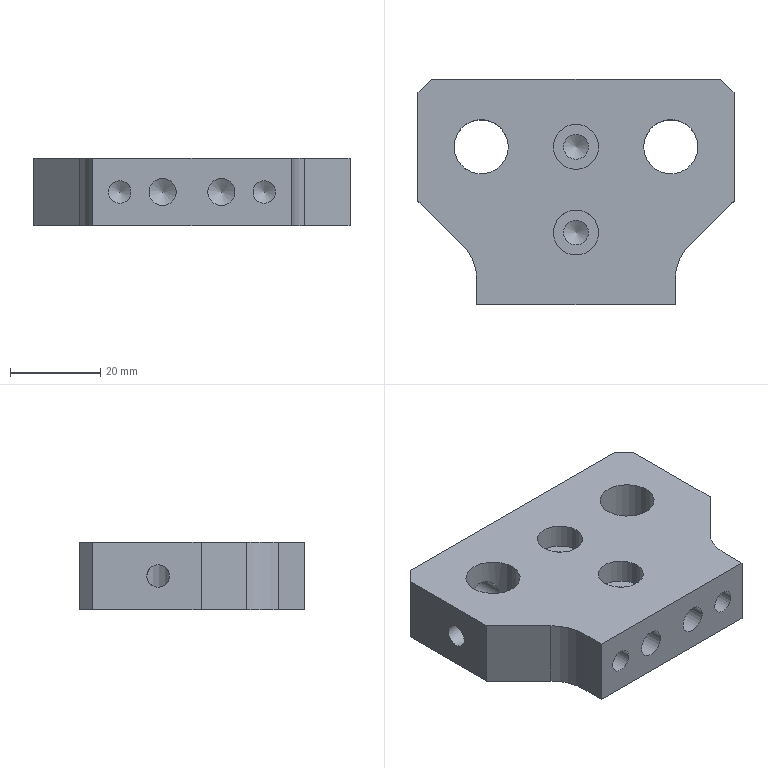Part | NX | features BREP 1 | 1 solid | 35 faces | box 70 x 50 x 15 mm | volume 39519 mm3 | cylinder 15 | plane 14 | cone 6 | commonest cylinder face diameters 5 x5 5.5 x2 6 x2 10 x2 12 x2 20 x2
STEP:
#1=CARTESIAN_POINT('',(35.,22.,0.));
#2=VERTEX_POINT('',#1);
#3=CARTESIAN_POINT('',(32.,25.,0.));
#4=VERTEX_POINT('',#3);
#5=CARTESIAN_POINT('',(35.,22.,0.));
#6=DIRECTION('',(-0.7071,0.7071,0.));
#7=VECTOR('',#6,1000.);
#8=LINE('',#5,#7);
#9=EDGE_CURVE('',#2,#4,#8,.T.);
#10=ORIENTED_EDGE('',*,*,#9,.F.);
#11=CARTESIAN_POINT('',(35.,-2.,0.));
#12=VERTEX_POINT('',#11);
#13=CARTESIAN_POINT('',(35.,0.,0.));
#14=DIRECTION('',(0.,1.,0.));
#15=VECTOR('',#14,1000.);
#16=LINE('',#13,#15);
#17=EDGE_CURVE('',#12,#2,#16,.T.);
#18=ORIENTED_EDGE('',*,*,#17,.F.);
#19=CARTESIAN_POINT('',(24.929,-12.071,0.));
#20=VERTEX_POINT('',#19);
#21=CARTESIAN_POINT('',(24.929,-12.071,0.));
#22=DIRECTION('',(0.7071,0.7071,0.));
#23=VECTOR('',#22,1000.);
#24=LINE('',#21,#23);
#25=EDGE_CURVE('',#20,#12,#24,.T.);
#26=ORIENTED_EDGE('',*,*,#25,.F.);
#27=CARTESIAN_POINT('',(22.,-19.142,0.));
#28=VERTEX_POINT('',#27);
#29=CARTESIAN_POINT('',(32.,-19.142,0.));
#30=DIRECTION('',(0.,0.,-1.));
#31=DIRECTION('',(1.,0.,0.));
#32=AXIS2_PLACEMENT_3D('',#29,#30,#31);
#33=CIRCLE('',#32,10.);
#34=EDGE_CURVE('',#28,#20,#33,.T.);
#35=ORIENTED_EDGE('',*,*,#34,.F.);
#36=CARTESIAN_POINT('',(22.,-25.,0.));
#37=VERTEX_POINT('',#36);
#38=CARTESIAN_POINT('',(22.,0.,0.));
#39=DIRECTION('',(0.,1.,0.));
#40=VECTOR('',#39,1000.);
#41=LINE('',#38,#40);
#42=EDGE_CURVE('',#37,#28,#41,.T.);
#43=ORIENTED_EDGE('',*,*,#42,.F.);
#44=CARTESIAN_POINT('',(-22.,-25.,0.));
#45=VERTEX_POINT('',#44);
#46=CARTESIAN_POINT('',(0.,-25.,0.));
#47=DIRECTION('',(1.,0.,0.));
#48=VECTOR('',#47,1000.);
#49=LINE('',#46,#48);
#50=EDGE_CURVE('',#45,#37,#49,.T.);
#51=ORIENTED_EDGE('',*,*,#50,.F.);
#52=CARTESIAN_POINT('',(-22.,-19.142,0.));
#53=VERTEX_POINT('',#52);
#54=CARTESIAN_POINT('',(-22.,0.,0.));
#55=DIRECTION('',(0.,-1.,0.));
#56=VECTOR('',#55,1000.);
#57=LINE('',#54,#56);
#58=EDGE_CURVE('',#53,#45,#57,.T.);
#59=ORIENTED_EDGE('',*,*,#58,.F.);
#60=CARTESIAN_POINT('',(-24.929,-12.071,0.));
#61=VERTEX_POINT('',#60);
#62=CARTESIAN_POINT('',(-32.,-19.142,0.));
#63=DIRECTION('',(0.,0.,-1.));
#64=DIRECTION('',(1.,0.,0.));
#65=AXIS2_PLACEMENT_3D('',#62,#63,#64);
#66=CIRCLE('',#65,10.);
#67=EDGE_CURVE('',#61,#53,#66,.T.);
#68=ORIENTED_EDGE('',*,*,#67,.F.);
#69=CARTESIAN_POINT('',(-35.,-2.,0.));
#70=VERTEX_POINT('',#69);
#71=CARTESIAN_POINT('',(-35.,-2.,0.));
#72=DIRECTION('',(0.7071,-0.7071,0.));
#73=VECTOR('',#72,1000.);
#74=LINE('',#71,#73);
#75=EDGE_CURVE('',#70,#61,#74,.T.);
#76=ORIENTED_EDGE('',*,*,#75,.F.);
#77=CARTESIAN_POINT('',(-35.,22.,0.));
#78=VERTEX_POINT('',#77);
#79=CARTESIAN_POINT('',(-35.,0.,0.));
#80=DIRECTION('',(0.,-1.,0.));
#81=VECTOR('',#80,1000.);
#82=LINE('',#79,#81);
#83=EDGE_CURVE('',#78,#70,#82,.T.);
#84=ORIENTED_EDGE('',*,*,#83,.F.);
#85=CARTESIAN_POINT('',(-32.,25.,0.));
#86=VERTEX_POINT('',#85);
#87=CARTESIAN_POINT('',(-32.,25.,0.));
#88=DIRECTION('',(-0.7071,-0.7071,0.));
#89=VECTOR('',#88,1000.);
#90=LINE('',#87,#89);
#91=EDGE_CURVE('',#86,#78,#90,.T.);
#92=ORIENTED_EDGE('',*,*,#91,.F.);
#93=CARTESIAN_POINT('',(0.,25.,0.));
#94=DIRECTION('',(-1.,0.,0.));
#95=VECTOR('',#94,1000.);
#96=LINE('',#93,#95);
#97=EDGE_CURVE('',#4,#86,#96,.T.);
#98=ORIENTED_EDGE('',*,*,#97,.F.);
#99=EDGE_LOOP('',(#10,#18,#26,#35,#43,#51,#59,#68,#76,#84,#92,#98));
#100=FACE_BOUND('',#99,.T.);
#101=CARTESIAN_POINT('',(15.,10.,0.));
#102=VERTEX_POINT('',#101);
#103=CARTESIAN_POINT('',(21.,10.,0.));
#104=DIRECTION('',(0.,0.,-1.));
#105=DIRECTION('',(-1.,0.,0.));
#106=AXIS2_PLACEMENT_3D('',#103,#104,#105);
#107=CIRCLE('',#106,6.);
#108=EDGE_CURVE('',#102,#102,#107,.T.);
#109=ORIENTED_EDGE('',*,*,#108,.F.);
#110=EDGE_LOOP('',(#109));
#111=FACE_BOUND('',#110,.T.);
#112=CARTESIAN_POINT('',(-27.,10.,0.));
#113=VERTEX_POINT('',#112);
#114=CARTESIAN_POINT('',(-21.,10.,0.));
#115=DIRECTION('',(0.,0.,-1.));
#116=DIRECTION('',(-1.,0.,0.));
#117=AXIS2_PLACEMENT_3D('',#114,#115,#116);
#118=CIRCLE('',#117,6.);
#119=EDGE_CURVE('',#113,#113,#118,.T.);
#120=ORIENTED_EDGE('',*,*,#119,.F.);
#121=EDGE_LOOP('',(#120));
#122=FACE_BOUND('',#121,.T.);
#123=CARTESIAN_POINT('',(0.,0.,0.));
#124=DIRECTION('',(0.,0.,1.));
#125=DIRECTION('',(-1.,0.,0.));
#126=AXIS2_PLACEMENT_3D('',#123,#124,#125);
#127=PLANE('',#126);
#128=ADVANCED_FACE('',(#100,#111,#122),#127,.F.);
#129=CARTESIAN_POINT('',(32.,25.,15.));
#130=VERTEX_POINT('',#129);
#131=CARTESIAN_POINT('',(32.,25.,15.));
#132=DIRECTION('',(0.,0.,1.));
#133=VECTOR('',#132,1000.);
#134=LINE('',#131,#133);
#135=EDGE_CURVE('',#4,#130,#134,.T.);
#136=ORIENTED_EDGE('',*,*,#135,.F.);
#137=ORIENTED_EDGE('',*,*,#97,.T.);
#138=CARTESIAN_POINT('',(-32.,25.,15.));
#139=VERTEX_POINT('',#138);
#140=CARTESIAN_POINT('',(-32.,25.,15.));
#141=DIRECTION('',(0.,0.,-1.));
#142=VECTOR('',#141,1000.);
#143=LINE('',#140,#142);
#144=EDGE_CURVE('',#139,#86,#143,.T.);
#145=ORIENTED_EDGE('',*,*,#144,.F.);
#146=CARTESIAN_POINT('',(-35.,25.,15.));
#147=DIRECTION('',(-1.,0.,0.));
#148=VECTOR('',#147,1000.);
#149=LINE('',#146,#148);
#150=EDGE_CURVE('',#130,#139,#149,.T.);
#151=ORIENTED_EDGE('',*,*,#150,.F.);
#152=EDGE_LOOP('',(#136,#137,#145,#151));
#153=FACE_BOUND('',#152,.T.);
#154=CARTESIAN_POINT('',(18.5,25.,10.));
#155=VERTEX_POINT('',#154);
#156=CARTESIAN_POINT('',(18.5,25.,7.5));
#157=DIRECTION('',(0.,1.,0.));
#158=DIRECTION('',(0.,0.,1.));
#159=AXIS2_PLACEMENT_3D('',#156,#157,#158);
#160=CIRCLE('',#159,2.5);
#161=EDGE_CURVE('',#155,#155,#160,.T.);
#162=ORIENTED_EDGE('',*,*,#161,.F.);
#163=EDGE_LOOP('',(#162));
#164=FACE_BOUND('',#163,.T.);
#165=CARTESIAN_POINT('',(-18.5,25.,10.));
#166=VERTEX_POINT('',#165);
#167=CARTESIAN_POINT('',(-18.5,25.,7.5));
#168=DIRECTION('',(0.,1.,0.));
#169=DIRECTION('',(0.,0.,1.));
#170=AXIS2_PLACEMENT_3D('',#167,#168,#169);
#171=CIRCLE('',#170,2.5);
#172=EDGE_CURVE('',#166,#166,#171,.T.);
#173=ORIENTED_EDGE('',*,*,#172,.F.);
#174=EDGE_LOOP('',(#173));
#175=FACE_BOUND('',#174,.T.);
#176=CARTESIAN_POINT('',(-35.,25.,15.));
#177=DIRECTION('',(0.,-1.,0.));
#178=DIRECTION('',(0.,0.,1.));
#179=AXIS2_PLACEMENT_3D('',#176,#177,#178);
#180=PLANE('',#179);
#181=ADVANCED_FACE('',(#153,#164,#175),#180,.F.);
#182=CARTESIAN_POINT('',(35.,22.,15.));
#183=VERTEX_POINT('',#182);
#184=CARTESIAN_POINT('',(35.,22.,15.));
#185=DIRECTION('',(0.,0.,1.));
#186=VECTOR('',#185,1000.);
#187=LINE('',#184,#186);
#188=EDGE_CURVE('',#2,#183,#187,.T.);
#189=ORIENTED_EDGE('',*,*,#188,.F.);
#190=ORIENTED_EDGE('',*,*,#9,.T.);
#191=ORIENTED_EDGE('',*,*,#135,.T.);
#192=CARTESIAN_POINT('',(32.,25.,15.));
#193=DIRECTION('',(-0.7071,0.7071,0.));
#194=VECTOR('',#193,1000.);
#195=LINE('',#192,#194);
#196=EDGE_CURVE('',#183,#130,#195,.T.);
#197=ORIENTED_EDGE('',*,*,#196,.F.);
#198=EDGE_LOOP('',(#189,#190,#191,#197));
#199=FACE_BOUND('',#198,.T.);
#200=CARTESIAN_POINT('',(32.,25.,15.));
#201=DIRECTION('',(-0.7071,-0.7071,0.));
#202=DIRECTION('',(-0.7071,0.7071,0.));
#203=AXIS2_PLACEMENT_3D('',#200,#201,#202);
#204=PLANE('',#203);
#205=ADVANCED_FACE('',(#199),#204,.F.);
#206=ORIENTED_EDGE('',*,*,#188,.T.);
#207=CARTESIAN_POINT('',(35.,-2.,15.));
#208=VERTEX_POINT('',#207);
#209=CARTESIAN_POINT('',(35.,25.,15.));
#210=DIRECTION('',(0.,1.,0.));
#211=VECTOR('',#210,1000.);
#212=LINE('',#209,#211);
#213=EDGE_CURVE('',#208,#183,#212,.T.);
#214=ORIENTED_EDGE('',*,*,#213,.F.);
#215=CARTESIAN_POINT('',(35.,-2.,15.));
#216=DIRECTION('',(0.,0.,1.));
#217=VECTOR('',#216,1000.);
#218=LINE('',#215,#217);
#219=EDGE_CURVE('',#12,#208,#218,.T.);
#220=ORIENTED_EDGE('',*,*,#219,.F.);
#221=ORIENTED_EDGE('',*,*,#17,.T.);
#222=EDGE_LOOP('',(#206,#214,#220,#221));
#223=FACE_BOUND('',#222,.T.);
#224=CARTESIAN_POINT('',(35.,25.,15.));
#225=DIRECTION('',(-1.,0.,0.));
#226=DIRECTION('',(0.,1.,0.));
#227=AXIS2_PLACEMENT_3D('',#224,#225,#226);
#228=PLANE('',#227);
#229=ADVANCED_FACE('',(#223),#228,.F.);
#230=CARTESIAN_POINT('',(24.929,-12.071,15.));
#231=VERTEX_POINT('',#230);
#232=CARTESIAN_POINT('',(24.929,-12.071,15.));
#233=DIRECTION('',(0.,0.,1.));
#234=VECTOR('',#233,1000.);
#235=LINE('',#232,#234);
#236=EDGE_CURVE('',#20,#231,#235,.T.);
#237=ORIENTED_EDGE('',*,*,#236,.F.);
#238=ORIENTED_EDGE('',*,*,#25,.T.);
#239=ORIENTED_EDGE('',*,*,#219,.T.);
#240=CARTESIAN_POINT('',(22.,-15.,15.));
#241=DIRECTION('',(0.7071,0.7071,0.));
#242=VECTOR('',#241,1000.);
#243=LINE('',#240,#242);
#244=EDGE_CURVE('',#231,#208,#243,.T.);
#245=ORIENTED_EDGE('',*,*,#244,.F.);
#246=EDGE_LOOP('',(#237,#238,#239,#245));
#247=FACE_BOUND('',#246,.T.);
#248=CARTESIAN_POINT('',(22.,-15.,15.));
#249=DIRECTION('',(-0.7071,0.7071,0.));
#250=DIRECTION('',(0.7071,0.7071,0.));
#251=AXIS2_PLACEMENT_3D('',#248,#249,#250);
#252=PLANE('',#251);
#253=ADVANCED_FACE('',(#247),#252,.F.);
#254=CARTESIAN_POINT('',(22.,-19.142,15.));
#255=VERTEX_POINT('',#254);
#256=CARTESIAN_POINT('',(22.,-19.142,15.));
#257=DIRECTION('',(0.,0.,1.));
#258=VECTOR('',#257,1000.);
#259=LINE('',#256,#258);
#260=EDGE_CURVE('',#28,#255,#259,.T.);
#261=ORIENTED_EDGE('',*,*,#260,.F.);
#262=ORIENTED_EDGE('',*,*,#34,.T.);
#263=ORIENTED_EDGE('',*,*,#236,.T.);
#264=CARTESIAN_POINT('',(32.,-19.142,15.));
#265=DIRECTION('',(0.,0.,-1.));
#266=DIRECTION('',(1.,0.,0.));
#267=AXIS2_PLACEMENT_3D('',#264,#265,#266);
#268=CIRCLE('',#267,10.);
#269=EDGE_CURVE('',#255,#231,#268,.T.);
#270=ORIENTED_EDGE('',*,*,#269,.F.);
#271=EDGE_LOOP('',(#261,#262,#263,#270));
#272=FACE_BOUND('',#271,.T.);
#273=CARTESIAN_POINT('',(32.,-19.142,15.));
#274=DIRECTION('',(0.,0.,1.));
#275=DIRECTION('',(-1.,0.,0.));
#276=AXIS2_PLACEMENT_3D('',#273,#274,#275);
#277=CYLINDRICAL_SURFACE('',#276,10.);
#278=ADVANCED_FACE('',(#272),#277,.F.);
#279=ORIENTED_EDGE('',*,*,#260,.T.);
#280=CARTESIAN_POINT('',(22.,-25.,15.));
#281=VERTEX_POINT('',#280);
#282=CARTESIAN_POINT('',(22.,-25.,15.));
#283=DIRECTION('',(0.,1.,0.));
#284=VECTOR('',#283,1000.);
#285=LINE('',#282,#284);
#286=EDGE_CURVE('',#281,#255,#285,.T.);
#287=ORIENTED_EDGE('',*,*,#286,.F.);
#288=CARTESIAN_POINT('',(22.,-25.,15.));
#289=DIRECTION('',(0.,0.,1.));
#290=VECTOR('',#289,1000.);
#291=LINE('',#288,#290);
#292=EDGE_CURVE('',#37,#281,#291,.T.);
#293=ORIENTED_EDGE('',*,*,#292,.F.);
#294=ORIENTED_EDGE('',*,*,#42,.T.);
#295=EDGE_LOOP('',(#279,#287,#293,#294));
#296=FACE_BOUND('',#295,.T.);
#297=CARTESIAN_POINT('',(22.,-25.,15.));
#298=DIRECTION('',(-1.,0.,0.));
#299=DIRECTION('',(0.,1.,0.));
#300=AXIS2_PLACEMENT_3D('',#297,#298,#299);
#301=PLANE('',#300);
#302=ADVANCED_FACE('',(#296),#301,.F.);
#303=ORIENTED_EDGE('',*,*,#50,.T.);
#304=ORIENTED_EDGE('',*,*,#292,.T.);
#305=CARTESIAN_POINT('',(-22.,-25.,15.));
#306=VERTEX_POINT('',#305);
#307=CARTESIAN_POINT('',(-35.,-25.,15.));
#308=DIRECTION('',(1.,0.,0.));
#309=VECTOR('',#308,1000.);
#310=LINE('',#307,#309);
#311=EDGE_CURVE('',#306,#281,#310,.T.);
#312=ORIENTED_EDGE('',*,*,#311,.F.);
#313=CARTESIAN_POINT('',(-22.,-25.,15.));
#314=DIRECTION('',(0.,0.,1.));
#315=VECTOR('',#314,1000.);
#316=LINE('',#313,#315);
#317=EDGE_CURVE('',#45,#306,#316,.T.);
#318=ORIENTED_EDGE('',*,*,#317,.F.);
#319=EDGE_LOOP('',(#303,#304,#312,#318));
#320=FACE_BOUND('',#319,.T.);
#321=CARTESIAN_POINT('',(16.,-25.,5.));
#322=VERTEX_POINT('',#321);
#323=CARTESIAN_POINT('',(16.,-25.,7.5));
#324=DIRECTION('',(0.,-1.,0.));
#325=DIRECTION('',(0.,0.,-1.));
#326=AXIS2_PLACEMENT_3D('',#323,#324,#325);
#327=CIRCLE('',#326,2.5);
#328=EDGE_CURVE('',#322,#322,#327,.T.);
#329=ORIENTED_EDGE('',*,*,#328,.F.);
#330=EDGE_LOOP('',(#329));
#331=FACE_BOUND('',#330,.T.);
#332=CARTESIAN_POINT('',(-16.,-25.,5.));
#333=VERTEX_POINT('',#332);
#334=CARTESIAN_POINT('',(-16.,-25.,7.5));
#335=DIRECTION('',(0.,-1.,0.));
#336=DIRECTION('',(0.,0.,-1.));
#337=AXIS2_PLACEMENT_3D('',#334,#335,#336);
#338=CIRCLE('',#337,2.5);
#339=EDGE_CURVE('',#333,#333,#338,.T.);
#340=ORIENTED_EDGE('',*,*,#339,.F.);
#341=EDGE_LOOP('',(#340));
#342=FACE_BOUND('',#341,.T.);
#343=CARTESIAN_POINT('',(6.5,-25.,4.5));
#344=VERTEX_POINT('',#343);
#345=CARTESIAN_POINT('',(6.5,-25.,7.5));
#346=DIRECTION('',(0.,-1.,0.));
#347=DIRECTION('',(0.,0.,-1.));
#348=AXIS2_PLACEMENT_3D('',#345,#346,#347);
#349=CIRCLE('',#348,3.);
#350=EDGE_CURVE('',#344,#344,#349,.T.);
#351=ORIENTED_EDGE('',*,*,#350,.F.);
#352=EDGE_LOOP('',(#351));
#353=FACE_BOUND('',#352,.T.);
#354=CARTESIAN_POINT('',(-6.5,-25.,4.5));
#355=VERTEX_POINT('',#354);
#356=CARTESIAN_POINT('',(-6.5,-25.,7.5));
#357=DIRECTION('',(0.,-1.,0.));
#358=DIRECTION('',(0.,0.,-1.));
#359=AXIS2_PLACEMENT_3D('',#356,#357,#358);
#360=CIRCLE('',#359,3.);
#361=EDGE_CURVE('',#355,#355,#360,.T.);
#362=ORIENTED_EDGE('',*,*,#361,.F.);
#363=EDGE_LOOP('',(#362));
#364=FACE_BOUND('',#363,.T.);
#365=CARTESIAN_POINT('',(-35.,-25.,15.));
#366=DIRECTION('',(0.,1.,0.));
#367=DIRECTION('',(0.,0.,-1.));
#368=AXIS2_PLACEMENT_3D('',#365,#366,#367);
#369=PLANE('',#368);
#370=ADVANCED_FACE('',(#320,#331,#342,#353,#364),#369,.F.);
#371=ORIENTED_EDGE('',*,*,#58,.T.);
#372=ORIENTED_EDGE('',*,*,#317,.T.);
#373=CARTESIAN_POINT('',(-22.,-19.142,15.));
#374=VERTEX_POINT('',#373);
#375=CARTESIAN_POINT('',(-22.,-25.,15.));
#376=DIRECTION('',(0.,1.,0.));
#377=VECTOR('',#376,1000.);
#378=LINE('',#375,#377);
#379=EDGE_CURVE('',#306,#374,#378,.T.);
#380=ORIENTED_EDGE('',*,*,#379,.T.);
#381=CARTESIAN_POINT('',(-22.,-19.142,15.));
#382=DIRECTION('',(0.,0.,-1.));
#383=VECTOR('',#382,1000.);
#384=LINE('',#381,#383);
#385=EDGE_CURVE('',#374,#53,#384,.T.);
#386=ORIENTED_EDGE('',*,*,#385,.T.);
#387=EDGE_LOOP('',(#371,#372,#380,#386));
#388=FACE_BOUND('',#387,.T.);
#389=CARTESIAN_POINT('',(-22.,-25.,15.));
#390=DIRECTION('',(-1.,0.,0.));
#391=DIRECTION('',(0.,1.,0.));
#392=AXIS2_PLACEMENT_3D('',#389,#390,#391);
#393=PLANE('',#392);
#394=ADVANCED_FACE('',(#388),#393,.T.);
#395=CARTESIAN_POINT('',(-24.929,-12.071,15.));
#396=VERTEX_POINT('',#395);
#397=CARTESIAN_POINT('',(-24.929,-12.071,15.));
#398=DIRECTION('',(0.,0.,1.));
#399=VECTOR('',#398,1000.);
#400=LINE('',#397,#399);
#401=EDGE_CURVE('',#61,#396,#400,.T.);
#402=ORIENTED_EDGE('',*,*,#401,.F.);
#403=ORIENTED_EDGE('',*,*,#67,.T.);
#404=ORIENTED_EDGE('',*,*,#385,.F.);
#405=CARTESIAN_POINT('',(-32.,-19.142,15.));
#406=DIRECTION('',(0.,0.,-1.));
#407=DIRECTION('',(1.,0.,0.));
#408=AXIS2_PLACEMENT_3D('',#405,#406,#407);
#409=CIRCLE('',#408,10.);
#410=EDGE_CURVE('',#396,#374,#409,.T.);
#411=ORIENTED_EDGE('',*,*,#410,.F.);
#412=EDGE_LOOP('',(#402,#403,#404,#411));
#413=FACE_BOUND('',#412,.T.);
#414=CARTESIAN_POINT('',(-32.,-19.142,15.));
#415=DIRECTION('',(0.,0.,1.));
#416=DIRECTION('',(-1.,0.,0.));
#417=AXIS2_PLACEMENT_3D('',#414,#415,#416);
#418=CYLINDRICAL_SURFACE('',#417,10.);
#419=ADVANCED_FACE('',(#413),#418,.F.);
#420=CARTESIAN_POINT('',(-35.,-2.,15.));
#421=VERTEX_POINT('',#420);
#422=CARTESIAN_POINT('',(-22.,-15.,15.));
#423=DIRECTION('',(-0.7071,0.7071,0.));
#424=VECTOR('',#423,1000.);
#425=LINE('',#422,#424);
#426=EDGE_CURVE('',#396,#421,#425,.T.);
#427=ORIENTED_EDGE('',*,*,#426,.T.);
#428=CARTESIAN_POINT('',(-35.,-2.,15.));
#429=DIRECTION('',(0.,0.,-1.));
#430=VECTOR('',#429,1000.);
#431=LINE('',#428,#430);
#432=EDGE_CURVE('',#421,#70,#431,.T.);
#433=ORIENTED_EDGE('',*,*,#432,.T.);
#434=ORIENTED_EDGE('',*,*,#75,.T.);
#435=ORIENTED_EDGE('',*,*,#401,.T.);
#436=EDGE_LOOP('',(#427,#433,#434,#435));
#437=FACE_BOUND('',#436,.T.);
#438=CARTESIAN_POINT('',(-22.,-15.,15.));
#439=DIRECTION('',(-0.7071,-0.7071,0.));
#440=DIRECTION('',(-0.7071,0.7071,0.));
#441=AXIS2_PLACEMENT_3D('',#438,#439,#440);
#442=PLANE('',#441);
#443=ADVANCED_FACE('',(#437),#442,.T.);
#444=CARTESIAN_POINT('',(-35.,22.,15.));
#445=VERTEX_POINT('',#444);
#446=CARTESIAN_POINT('',(-35.,22.,15.));
#447=DIRECTION('',(0.,0.,1.));
#448=VECTOR('',#447,1000.);
#449=LINE('',#446,#448);
#450=EDGE_CURVE('',#78,#445,#449,.T.);
#451=ORIENTED_EDGE('',*,*,#450,.F.);
#452=ORIENTED_EDGE('',*,*,#83,.T.);
#453=ORIENTED_EDGE('',*,*,#432,.F.);
#454=CARTESIAN_POINT('',(-35.,25.,15.));
#455=DIRECTION('',(0.,-1.,0.));
#456=VECTOR('',#455,1000.);
#457=LINE('',#454,#456);
#458=EDGE_CURVE('',#445,#421,#457,.T.);
#459=ORIENTED_EDGE('',*,*,#458,.F.);
#460=EDGE_LOOP('',(#451,#452,#453,#459));
#461=FACE_BOUND('',#460,.T.);
#462=CARTESIAN_POINT('',(-35.,7.5,10.));
#463=VERTEX_POINT('',#462);
#464=CARTESIAN_POINT('',(-35.,7.5,7.5));
#465=DIRECTION('',(-1.,0.,0.));
#466=DIRECTION('',(0.,0.,1.));
#467=AXIS2_PLACEMENT_3D('',#464,#465,#466);
#468=CIRCLE('',#467,2.5);
#469=EDGE_CURVE('',#463,#463,#468,.T.);
#470=ORIENTED_EDGE('',*,*,#469,.F.);
#471=EDGE_LOOP('',(#470));
#472=FACE_BOUND('',#471,.T.);
#473=CARTESIAN_POINT('',(-35.,25.,15.));
#474=DIRECTION('',(1.,0.,0.));
#475=DIRECTION('',(0.,-1.,0.));
#476=AXIS2_PLACEMENT_3D('',#473,#474,#475);
#477=PLANE('',#476);
#478=ADVANCED_FACE('',(#461,#472),#477,.F.);
#479=ORIENTED_EDGE('',*,*,#144,.T.);
#480=ORIENTED_EDGE('',*,*,#91,.T.);
#481=ORIENTED_EDGE('',*,*,#450,.T.);
#482=CARTESIAN_POINT('',(-35.,22.,15.));
#483=DIRECTION('',(-0.7071,-0.7071,0.));
#484=VECTOR('',#483,1000.);
#485=LINE('',#482,#484);
#486=EDGE_CURVE('',#139,#445,#485,.T.);
#487=ORIENTED_EDGE('',*,*,#486,.F.);
#488=EDGE_LOOP('',(#479,#480,#481,#487));
#489=FACE_BOUND('',#488,.T.);
#490=CARTESIAN_POINT('',(-35.,22.,15.));
#491=DIRECTION('',(0.7071,-0.7071,0.));
#492=DIRECTION('',(-0.7071,-0.7071,0.));
#493=AXIS2_PLACEMENT_3D('',#490,#491,#492);
#494=PLANE('',#493);
#495=ADVANCED_FACE('',(#489),#494,.F.);
#496=CARTESIAN_POINT('',(15.,10.,15.));
#497=VERTEX_POINT('',#496);
#498=CARTESIAN_POINT('',(21.,10.,15.));
#499=DIRECTION('',(0.,0.,-1.));
#500=DIRECTION('',(-1.,0.,0.));
#501=AXIS2_PLACEMENT_3D('',#498,#499,#500);
#502=CIRCLE('',#501,6.);
#503=EDGE_CURVE('',#497,#497,#502,.T.);
#504=ORIENTED_EDGE('',*,*,#503,.F.);
#505=EDGE_LOOP('',(#504));
#506=FACE_BOUND('',#505,.T.);
#507=CARTESIAN_POINT('',(18.5,15.454,5.));
#508=VERTEX_POINT('',#507);
#509=CARTESIAN_POINT('',(17.561,14.951,5.127));
#510=CARTESIAN_POINT('',(18.793,15.668,4.866));
#511=CARTESIAN_POINT('',(20.559,16.052,5.568));
#512=CARTESIAN_POINT('',(21.312,15.978,7.792));
#513=CARTESIAN_POINT('',(20.113,16.035,9.81));
#514=CARTESIAN_POINT('',(18.294,15.444,10.129));
#515=CARTESIAN_POINT('',(17.177,14.656,9.679));
#516=CARTESIAN_POINT('',(16.525,14.028,9.109));
#517=CARTESIAN_POINT('',(16.069,13.431,8.33));
#518=CARTESIAN_POINT('',(15.936,13.219,7.221));
#519=CARTESIAN_POINT('',(16.265,13.711,6.261));
#520=CARTESIAN_POINT('',(16.815,14.331,5.589));
#521=CARTESIAN_POINT('',(17.561,14.951,5.127));
#522=CARTESIAN_POINT('',(18.793,15.668,4.866));
#523=CARTESIAN_POINT('',(20.559,16.052,5.568));
#524=B_SPLINE_CURVE_WITH_KNOTS('',3,(#509,#510,#511,#512,#513,#514,#515,#516,#517,#518,#519,#520,#521,#522,#523),.UNSPECIFIED.,.T.,.F.,(1,1,1,1,1,1,1,1,1,1,1,1,1,1,1,1,1,1,1),(-0.00318,-0.00212,-0.00106,0.,0.00212,0.004239,0.006359,0.008479,0.009539,0.0106,0.01166,0.01272,0.01378,0.01484,0.0159,0.01696,0.01908,0.0212,0.02332),.UNSPECIFIED.);
#525=EDGE_CURVE('',#508,#508,#524,.T.);
#526=ORIENTED_EDGE('',*,*,#525,.F.);
#527=EDGE_LOOP('',(#526));
#528=FACE_BOUND('',#527,.T.);
#529=ORIENTED_EDGE('',*,*,#108,.T.);
#530=EDGE_LOOP('',(#529));
#531=FACE_BOUND('',#530,.T.);
#532=CARTESIAN_POINT('',(21.,10.,0.));
#533=DIRECTION('',(0.,0.,-1.));
#534=DIRECTION('',(1.,0.,0.));
#535=AXIS2_PLACEMENT_3D('',#532,#533,#534);
#536=CYLINDRICAL_SURFACE('',#535,6.);
#537=ADVANCED_FACE('',(#506,#528,#531),#536,.F.);
#538=CARTESIAN_POINT('',(-26.454,7.5,5.));
#539=VERTEX_POINT('',#538);
#540=CARTESIAN_POINT('',(-25.951,6.561,5.127));
#541=CARTESIAN_POINT('',(-26.668,7.793,4.866));
#542=CARTESIAN_POINT('',(-27.052,9.559,5.568));
#543=CARTESIAN_POINT('',(-26.978,10.312,7.792));
#544=CARTESIAN_POINT('',(-27.035,9.113,9.81));
#545=CARTESIAN_POINT('',(-26.444,7.294,10.129));
#546=CARTESIAN_POINT('',(-25.656,6.177,9.679));
#547=CARTESIAN_POINT('',(-25.028,5.525,9.109));
#548=CARTESIAN_POINT('',(-24.431,5.069,8.33));
#549=CARTESIAN_POINT('',(-24.219,4.936,7.221));
#550=CARTESIAN_POINT('',(-24.711,5.265,6.261));
#551=CARTESIAN_POINT('',(-25.331,5.815,5.589));
#552=CARTESIAN_POINT('',(-25.951,6.561,5.127));
#553=CARTESIAN_POINT('',(-26.668,7.793,4.866));
#554=CARTESIAN_POINT('',(-27.052,9.559,5.568));
#555=B_SPLINE_CURVE_WITH_KNOTS('',3,(#540,#541,#542,#543,#544,#545,#546,#547,#548,#549,#550,#551,#552,#553,#554),.UNSPECIFIED.,.T.,.F.,(1,1,1,1,1,1,1,1,1,1,1,1,1,1,1,1,1,1,1),(-0.00318,-0.00212,-0.00106,0.,0.00212,0.004239,0.006359,0.008479,0.009539,0.0106,0.01166,0.01272,0.01378,0.01484,0.0159,0.01696,0.01908,0.0212,0.02332),.UNSPECIFIED.);
#556=EDGE_CURVE('',#539,#539,#555,.T.);
#557=ORIENTED_EDGE('',*,*,#556,.F.);
#558=EDGE_LOOP('',(#557));
#559=FACE_BOUND('',#558,.T.);
#560=CARTESIAN_POINT('',(-27.,10.,15.));
#561=VERTEX_POINT('',#560);
#562=CARTESIAN_POINT('',(-21.,10.,15.));
#563=DIRECTION('',(0.,0.,-1.));
#564=DIRECTION('',(-1.,0.,0.));
#565=AXIS2_PLACEMENT_3D('',#562,#563,#564);
#566=CIRCLE('',#565,6.);
#567=EDGE_CURVE('',#561,#561,#566,.T.);
#568=ORIENTED_EDGE('',*,*,#567,.F.);
#569=EDGE_LOOP('',(#568));
#570=FACE_BOUND('',#569,.T.);
#571=CARTESIAN_POINT('',(-18.5,15.454,5.));
#572=VERTEX_POINT('',#571);
#573=CARTESIAN_POINT('',(-20.564,16.052,5.57));
#574=CARTESIAN_POINT('',(-18.791,15.667,4.867));
#575=CARTESIAN_POINT('',(-17.564,14.953,5.126));
#576=CARTESIAN_POINT('',(-16.814,14.331,5.59));
#577=CARTESIAN_POINT('',(-16.268,13.714,6.256));
#578=CARTESIAN_POINT('',(-15.936,13.22,7.216));
#579=CARTESIAN_POINT('',(-16.067,13.428,8.324));
#580=CARTESIAN_POINT('',(-16.524,14.027,9.108));
#581=CARTESIAN_POINT('',(-17.173,14.652,9.676));
#582=CARTESIAN_POINT('',(-18.287,15.44,10.128));
#583=CARTESIAN_POINT('',(-20.104,16.034,9.816));
#584=CARTESIAN_POINT('',(-21.312,15.978,7.798));
#585=CARTESIAN_POINT('',(-20.564,16.052,5.57));
#586=CARTESIAN_POINT('',(-18.791,15.667,4.867));
#587=CARTESIAN_POINT('',(-17.564,14.953,5.126));
#588=B_SPLINE_CURVE_WITH_KNOTS('',3,(#573,#574,#575,#576,#577,#578,#579,#580,#581,#582,#583,#584,#585,#586,#587),.UNSPECIFIED.,.T.,.F.,(1,1,1,1,1,1,1,1,1,1,1,1,1,1,1,1,1,1,1),(-0.006348,-0.004232,-0.002116,0.,0.001058,0.002116,0.003174,0.004232,0.00529,0.006348,0.007406,0.008464,0.01058,0.0127,0.01481,0.01693,0.01799,0.01904,0.0201),.UNSPECIFIED.);
#589=EDGE_CURVE('',#572,#572,#588,.T.);
#590=ORIENTED_EDGE('',*,*,#589,.F.);
#591=EDGE_LOOP('',(#590));
#592=FACE_BOUND('',#591,.T.);
#593=ORIENTED_EDGE('',*,*,#119,.T.);
#594=EDGE_LOOP('',(#593));
#595=FACE_BOUND('',#594,.T.);
#596=CARTESIAN_POINT('',(-21.,10.,0.));
#597=DIRECTION('',(0.,0.,-1.));
#598=DIRECTION('',(1.,0.,0.));
#599=AXIS2_PLACEMENT_3D('',#596,#597,#598);
#600=CYLINDRICAL_SURFACE('',#599,6.);
#601=ADVANCED_FACE('',(#559,#570,#592,#595),#600,.F.);
#602=ORIENTED_EDGE('',*,*,#269,.T.);
#603=ORIENTED_EDGE('',*,*,#244,.T.);
#604=ORIENTED_EDGE('',*,*,#213,.T.);
#605=ORIENTED_EDGE('',*,*,#196,.T.);
#606=ORIENTED_EDGE('',*,*,#150,.T.);
#607=ORIENTED_EDGE('',*,*,#486,.T.);
#608=ORIENTED_EDGE('',*,*,#458,.T.);
#609=ORIENTED_EDGE('',*,*,#426,.F.);
#610=ORIENTED_EDGE('',*,*,#410,.T.);
#611=ORIENTED_EDGE('',*,*,#379,.F.);
#612=ORIENTED_EDGE('',*,*,#311,.T.);
#613=ORIENTED_EDGE('',*,*,#286,.T.);
#614=EDGE_LOOP('',(#602,#603,#604,#605,#606,#607,#608,#609,#610,#611,#612,#613));
#615=FACE_BOUND('',#614,.T.);
#616=ORIENTED_EDGE('',*,*,#503,.T.);
#617=EDGE_LOOP('',(#616));
#618=FACE_BOUND('',#617,.T.);
#619=ORIENTED_EDGE('',*,*,#567,.T.);
#620=EDGE_LOOP('',(#619));
#621=FACE_BOUND('',#620,.T.);
#622=CARTESIAN_POINT('',(5.,-9.,15.));
#623=VERTEX_POINT('',#622);
#624=CARTESIAN_POINT('',(0.,-9.,15.));
#625=DIRECTION('',(0.,0.,-1.));
#626=DIRECTION('',(1.,0.,0.));
#627=AXIS2_PLACEMENT_3D('',#624,#625,#626);
#628=CIRCLE('',#627,5.);
#629=EDGE_CURVE('',#623,#623,#628,.T.);
#630=ORIENTED_EDGE('',*,*,#629,.T.);
#631=EDGE_LOOP('',(#630));
#632=FACE_BOUND('',#631,.T.);
#633=CARTESIAN_POINT('',(5.,10.,15.));
#634=VERTEX_POINT('',#633);
#635=CARTESIAN_POINT('',(0.,10.,15.));
#636=DIRECTION('',(0.,0.,-1.));
#637=DIRECTION('',(1.,0.,0.));
#638=AXIS2_PLACEMENT_3D('',#635,#636,#637);
#639=CIRCLE('',#638,5.);
#640=EDGE_CURVE('',#634,#634,#639,.T.);
#641=ORIENTED_EDGE('',*,*,#640,.T.);
#642=EDGE_LOOP('',(#641));
#643=FACE_BOUND('',#642,.T.);
#644=CARTESIAN_POINT('',(0.,0.,15.));
#645=DIRECTION('',(0.,0.,1.));
#646=DIRECTION('',(-1.,0.,0.));
#647=AXIS2_PLACEMENT_3D('',#644,#645,#646);
#648=PLANE('',#647);
#649=ADVANCED_FACE('',(#615,#618,#621,#632,#643),#648,.T.);
#650=ORIENTED_EDGE('',*,*,#525,.T.);
#651=EDGE_LOOP('',(#650));
#652=FACE_BOUND('',#651,.T.);
#653=ORIENTED_EDGE('',*,*,#161,.T.);
#654=EDGE_LOOP('',(#653));
#655=FACE_BOUND('',#654,.T.);
#656=CARTESIAN_POINT('',(18.5,25.,7.5));
#657=DIRECTION('',(0.,1.,0.));
#658=DIRECTION('',(0.,0.,-1.));
#659=AXIS2_PLACEMENT_3D('',#656,#657,#658);
#660=CYLINDRICAL_SURFACE('',#659,2.5);
#661=ADVANCED_FACE('',(#652,#655),#660,.F.);
#662=ORIENTED_EDGE('',*,*,#589,.T.);
#663=EDGE_LOOP('',(#662));
#664=FACE_BOUND('',#663,.T.);
#665=ORIENTED_EDGE('',*,*,#172,.T.);
#666=EDGE_LOOP('',(#665));
#667=FACE_BOUND('',#666,.T.);
#668=CARTESIAN_POINT('',(-18.5,25.,7.5));
#669=DIRECTION('',(0.,1.,0.));
#670=DIRECTION('',(0.,0.,-1.));
#671=AXIS2_PLACEMENT_3D('',#668,#669,#670);
#672=CYLINDRICAL_SURFACE('',#671,2.5);
#673=ADVANCED_FACE('',(#664,#667),#672,.F.);
#674=CARTESIAN_POINT('',(16.,-10.,5.));
#675=VERTEX_POINT('',#674);
#676=CARTESIAN_POINT('',(16.,-10.,7.5));
#677=DIRECTION('',(0.,-1.,0.));
#678=DIRECTION('',(0.,0.,-1.));
#679=AXIS2_PLACEMENT_3D('',#676,#677,#678);
#680=CIRCLE('',#679,2.5);
#681=EDGE_CURVE('',#675,#675,#680,.T.);
#682=ORIENTED_EDGE('',*,*,#681,.F.);
#683=EDGE_LOOP('',(#682));
#684=FACE_BOUND('',#683,.T.);
#685=ORIENTED_EDGE('',*,*,#328,.T.);
#686=EDGE_LOOP('',(#685));
#687=FACE_BOUND('',#686,.T.);
#688=CARTESIAN_POINT('',(16.,-25.,7.5));
#689=DIRECTION('',(0.,-1.,0.));
#690=DIRECTION('',(0.,0.,1.));
#691=AXIS2_PLACEMENT_3D('',#688,#689,#690);
#692=CYLINDRICAL_SURFACE('',#691,2.5);
#693=ADVANCED_FACE('',(#684,#687),#692,.F.);
#694=CARTESIAN_POINT('',(-16.,-10.,5.));
#695=VERTEX_POINT('',#694);
#696=CARTESIAN_POINT('',(-16.,-10.,7.5));
#697=DIRECTION('',(0.,-1.,0.));
#698=DIRECTION('',(0.,0.,-1.));
#699=AXIS2_PLACEMENT_3D('',#696,#697,#698);
#700=CIRCLE('',#699,2.5);
#701=EDGE_CURVE('',#695,#695,#700,.T.);
#702=ORIENTED_EDGE('',*,*,#701,.F.);
#703=EDGE_LOOP('',(#702));
#704=FACE_BOUND('',#703,.T.);
#705=ORIENTED_EDGE('',*,*,#339,.T.);
#706=EDGE_LOOP('',(#705));
#707=FACE_BOUND('',#706,.T.);
#708=CARTESIAN_POINT('',(-16.,-25.,7.5));
#709=DIRECTION('',(0.,-1.,0.));
#710=DIRECTION('',(0.,0.,1.));
#711=AXIS2_PLACEMENT_3D('',#708,#709,#710);
#712=CYLINDRICAL_SURFACE('',#711,2.5);
#713=ADVANCED_FACE('',(#704,#707),#712,.F.);
#714=CARTESIAN_POINT('',(6.5,-13.,4.5));
#715=VERTEX_POINT('',#714);
#716=CARTESIAN_POINT('',(6.5,-13.,7.5));
#717=DIRECTION('',(0.,-1.,0.));
#718=DIRECTION('',(0.,0.,-1.));
#719=AXIS2_PLACEMENT_3D('',#716,#717,#718);
#720=CIRCLE('',#719,3.);
#721=EDGE_CURVE('',#715,#715,#720,.T.);
#722=ORIENTED_EDGE('',*,*,#721,.F.);
#723=EDGE_LOOP('',(#722));
#724=FACE_BOUND('',#723,.T.);
#725=ORIENTED_EDGE('',*,*,#350,.T.);
#726=EDGE_LOOP('',(#725));
#727=FACE_BOUND('',#726,.T.);
#728=CARTESIAN_POINT('',(6.5,-25.,7.5));
#729=DIRECTION('',(0.,-1.,0.));
#730=DIRECTION('',(0.,0.,1.));
#731=AXIS2_PLACEMENT_3D('',#728,#729,#730);
#732=CYLINDRICAL_SURFACE('',#731,3.);
#733=ADVANCED_FACE('',(#724,#727),#732,.F.);
#734=CARTESIAN_POINT('',(-6.5,-13.,4.5));
#735=VERTEX_POINT('',#734);
#736=CARTESIAN_POINT('',(-6.5,-13.,7.5));
#737=DIRECTION('',(0.,-1.,0.));
#738=DIRECTION('',(0.,0.,-1.));
#739=AXIS2_PLACEMENT_3D('',#736,#737,#738);
#740=CIRCLE('',#739,3.);
#741=EDGE_CURVE('',#735,#735,#740,.T.);
#742=ORIENTED_EDGE('',*,*,#741,.F.);
#743=EDGE_LOOP('',(#742));
#744=FACE_BOUND('',#743,.T.);
#745=ORIENTED_EDGE('',*,*,#361,.T.);
#746=EDGE_LOOP('',(#745));
#747=FACE_BOUND('',#746,.T.);
#748=CARTESIAN_POINT('',(-6.5,-25.,7.5));
#749=DIRECTION('',(0.,-1.,0.));
#750=DIRECTION('',(0.,0.,1.));
#751=AXIS2_PLACEMENT_3D('',#748,#749,#750);
#752=CYLINDRICAL_SURFACE('',#751,3.);
#753=ADVANCED_FACE('',(#744,#747),#752,.F.);
#754=ORIENTED_EDGE('',*,*,#556,.T.);
#755=EDGE_LOOP('',(#754));
#756=FACE_BOUND('',#755,.T.);
#757=ORIENTED_EDGE('',*,*,#469,.T.);
#758=EDGE_LOOP('',(#757));
#759=FACE_BOUND('',#758,.T.);
#760=CARTESIAN_POINT('',(-35.,7.5,7.5));
#761=DIRECTION('',(-1.,0.,0.));
#762=DIRECTION('',(0.,0.,-1.));
#763=AXIS2_PLACEMENT_3D('',#760,#761,#762);
#764=CYLINDRICAL_SURFACE('',#763,2.5);
#765=ADVANCED_FACE('',(#756,#759),#764,.F.);
#766=ORIENTED_EDGE('',*,*,#629,.F.);
#767=EDGE_LOOP('',(#766));
#768=FACE_BOUND('',#767,.T.);
#769=CARTESIAN_POINT('',(5.,-9.,9.6));
#770=VERTEX_POINT('',#769);
#771=CARTESIAN_POINT('',(0.,-9.,9.6));
#772=DIRECTION('',(0.,0.,1.));
#773=DIRECTION('',(1.,0.,0.));
#774=AXIS2_PLACEMENT_3D('',#771,#772,#773);
#775=CIRCLE('',#774,5.);
#776=EDGE_CURVE('',#770,#770,#775,.T.);
#777=ORIENTED_EDGE('',*,*,#776,.F.);
#778=EDGE_LOOP('',(#777));
#779=FACE_BOUND('',#778,.T.);
#780=CARTESIAN_POINT('',(0.,-9.,15.));
#781=DIRECTION('',(0.,0.,1.));
#782=DIRECTION('',(-1.,0.,0.));
#783=AXIS2_PLACEMENT_3D('',#780,#781,#782);
#784=CYLINDRICAL_SURFACE('',#783,5.);
#785=ADVANCED_FACE('',(#768,#779),#784,.F.);
#786=ORIENTED_EDGE('',*,*,#640,.F.);
#787=EDGE_LOOP('',(#786));
#788=FACE_BOUND('',#787,.T.);
#789=CARTESIAN_POINT('',(5.,10.,9.6));
#790=VERTEX_POINT('',#789);
#791=CARTESIAN_POINT('',(0.,10.,9.6));
#792=DIRECTION('',(0.,0.,1.));
#793=DIRECTION('',(1.,0.,0.));
#794=AXIS2_PLACEMENT_3D('',#791,#792,#793);
#795=CIRCLE('',#794,5.);
#796=EDGE_CURVE('',#790,#790,#795,.T.);
#797=ORIENTED_EDGE('',*,*,#796,.F.);
#798=EDGE_LOOP('',(#797));
#799=FACE_BOUND('',#798,.T.);
#800=CARTESIAN_POINT('',(0.,10.,15.));
#801=DIRECTION('',(0.,0.,1.));
#802=DIRECTION('',(-1.,0.,0.));
#803=AXIS2_PLACEMENT_3D('',#800,#801,#802);
#804=CYLINDRICAL_SURFACE('',#803,5.);
#805=ADVANCED_FACE('',(#788,#799),#804,.F.);
#806=CARTESIAN_POINT('',(16.,-8.498,7.5));
#807=VERTEX_POINT('',#806);
#808=VERTEX_LOOP('',#807);
#809=FACE_BOUND('',#808,.T.);
#810=ORIENTED_EDGE('',*,*,#681,.T.);
#811=EDGE_LOOP('',(#810));
#812=FACE_BOUND('',#811,.T.);
#813=CARTESIAN_POINT('',(16.,-10.,7.5));
#814=DIRECTION('',(0.,-1.,0.));
#815=DIRECTION('',(0.,0.,1.));
#816=AXIS2_PLACEMENT_3D('',#813,#814,#815);
#817=CONICAL_SURFACE('',#816,2.5,1.03);
#818=ADVANCED_FACE('',(#809,#812),#817,.F.);
#819=CARTESIAN_POINT('',(-16.,-8.498,7.5));
#820=VERTEX_POINT('',#819);
#821=VERTEX_LOOP('',#820);
#822=FACE_BOUND('',#821,.T.);
#823=ORIENTED_EDGE('',*,*,#701,.T.);
#824=EDGE_LOOP('',(#823));
#825=FACE_BOUND('',#824,.T.);
#826=CARTESIAN_POINT('',(-16.,-10.,7.5));
#827=DIRECTION('',(0.,-1.,0.));
#828=DIRECTION('',(0.,0.,1.));
#829=AXIS2_PLACEMENT_3D('',#826,#827,#828);
#830=CONICAL_SURFACE('',#829,2.5,1.03);
#831=ADVANCED_FACE('',(#822,#825),#830,.F.);
#832=CARTESIAN_POINT('',(6.5,-11.197,7.5));
#833=VERTEX_POINT('',#832);
#834=VERTEX_LOOP('',#833);
#835=FACE_BOUND('',#834,.T.);
#836=ORIENTED_EDGE('',*,*,#721,.T.);
#837=EDGE_LOOP('',(#836));
#838=FACE_BOUND('',#837,.T.);
#839=CARTESIAN_POINT('',(6.5,-13.,7.5));
#840=DIRECTION('',(0.,-1.,0.));
#841=DIRECTION('',(0.,0.,1.));
#842=AXIS2_PLACEMENT_3D('',#839,#840,#841);
#843=CONICAL_SURFACE('',#842,3.,1.03);
#844=ADVANCED_FACE('',(#835,#838),#843,.F.);
#845=CARTESIAN_POINT('',(-6.5,-11.197,7.5));
#846=VERTEX_POINT('',#845);
#847=VERTEX_LOOP('',#846);
#848=FACE_BOUND('',#847,.T.);
#849=ORIENTED_EDGE('',*,*,#741,.T.);
#850=EDGE_LOOP('',(#849));
#851=FACE_BOUND('',#850,.T.);
#852=CARTESIAN_POINT('',(-6.5,-13.,7.5));
#853=DIRECTION('',(0.,-1.,0.));
#854=DIRECTION('',(0.,0.,1.));
#855=AXIS2_PLACEMENT_3D('',#852,#853,#854);
#856=CONICAL_SURFACE('',#855,3.,1.03);
#857=ADVANCED_FACE('',(#848,#851),#856,.F.);
#858=ORIENTED_EDGE('',*,*,#776,.T.);
#859=EDGE_LOOP('',(#858));
#860=FACE_BOUND('',#859,.T.);
#861=CARTESIAN_POINT('',(2.75,-9.,9.6));
#862=VERTEX_POINT('',#861);
#863=CARTESIAN_POINT('',(0.,-9.,9.6));
#864=DIRECTION('',(0.,0.,1.));
#865=DIRECTION('',(1.,0.,0.));
#866=AXIS2_PLACEMENT_3D('',#863,#864,#865);
#867=CIRCLE('',#866,2.75);
#868=EDGE_CURVE('',#862,#862,#867,.T.);
#869=ORIENTED_EDGE('',*,*,#868,.F.);
#870=EDGE_LOOP('',(#869));
#871=FACE_BOUND('',#870,.T.);
#872=CARTESIAN_POINT('',(2.75,-9.,9.6));
#873=DIRECTION('',(0.,0.,-1.));
#874=DIRECTION('',(1.,0.,0.));
#875=AXIS2_PLACEMENT_3D('',#872,#873,#874);
#876=PLANE('',#875);
#877=ADVANCED_FACE('',(#860,#871),#876,.F.);
#878=ORIENTED_EDGE('',*,*,#796,.T.);
#879=EDGE_LOOP('',(#878));
#880=FACE_BOUND('',#879,.T.);
#881=CARTESIAN_POINT('',(2.75,10.,9.6));
#882=VERTEX_POINT('',#881);
#883=CARTESIAN_POINT('',(0.,10.,9.6));
#884=DIRECTION('',(0.,0.,1.));
#885=DIRECTION('',(1.,0.,0.));
#886=AXIS2_PLACEMENT_3D('',#883,#884,#885);
#887=CIRCLE('',#886,2.75);
#888=EDGE_CURVE('',#882,#882,#887,.T.);
#889=ORIENTED_EDGE('',*,*,#888,.F.);
#890=EDGE_LOOP('',(#889));
#891=FACE_BOUND('',#890,.T.);
#892=CARTESIAN_POINT('',(2.75,10.,9.6));
#893=DIRECTION('',(0.,0.,-1.));
#894=DIRECTION('',(1.,0.,0.));
#895=AXIS2_PLACEMENT_3D('',#892,#893,#894);
#896=PLANE('',#895);
#897=ADVANCED_FACE('',(#880,#891),#896,.F.);
#898=CARTESIAN_POINT('',(2.75,-9.,2.6));
#899=VERTEX_POINT('',#898);
#900=CARTESIAN_POINT('',(0.,-9.,2.6));
#901=DIRECTION('',(0.,0.,1.));
#902=DIRECTION('',(1.,0.,0.));
#903=AXIS2_PLACEMENT_3D('',#900,#901,#902);
#904=CIRCLE('',#903,2.75);
#905=EDGE_CURVE('',#899,#899,#904,.T.);
#906=ORIENTED_EDGE('',*,*,#905,.F.);
#907=EDGE_LOOP('',(#906));
#908=FACE_BOUND('',#907,.T.);
#909=ORIENTED_EDGE('',*,*,#868,.T.);
#910=EDGE_LOOP('',(#909));
#911=FACE_BOUND('',#910,.T.);
#912=CARTESIAN_POINT('',(0.,-9.,15.));
#913=DIRECTION('',(0.,0.,1.));
#914=DIRECTION('',(-1.,0.,0.));
#915=AXIS2_PLACEMENT_3D('',#912,#913,#914);
#916=CYLINDRICAL_SURFACE('',#915,2.75);
#917=ADVANCED_FACE('',(#908,#911),#916,.F.);
#918=CARTESIAN_POINT('',(2.75,10.,2.6));
#919=VERTEX_POINT('',#918);
#920=CARTESIAN_POINT('',(0.,10.,2.6));
#921=DIRECTION('',(0.,0.,1.));
#922=DIRECTION('',(1.,0.,0.));
#923=AXIS2_PLACEMENT_3D('',#920,#921,#922);
#924=CIRCLE('',#923,2.75);
#925=EDGE_CURVE('',#919,#919,#924,.T.);
#926=ORIENTED_EDGE('',*,*,#925,.F.);
#927=EDGE_LOOP('',(#926));
#928=FACE_BOUND('',#927,.T.);
#929=ORIENTED_EDGE('',*,*,#888,.T.);
#930=EDGE_LOOP('',(#929));
#931=FACE_BOUND('',#930,.T.);
#932=CARTESIAN_POINT('',(0.,10.,15.));
#933=DIRECTION('',(0.,0.,1.));
#934=DIRECTION('',(-1.,0.,0.));
#935=AXIS2_PLACEMENT_3D('',#932,#933,#934);
#936=CYLINDRICAL_SURFACE('',#935,2.75);
#937=ADVANCED_FACE('',(#928,#931),#936,.F.);
#938=CARTESIAN_POINT('',(0.,-9.,0.9476));
#939=VERTEX_POINT('',#938);
#940=VERTEX_LOOP('',#939);
#941=FACE_BOUND('',#940,.T.);
#942=ORIENTED_EDGE('',*,*,#905,.T.);
#943=EDGE_LOOP('',(#942));
#944=FACE_BOUND('',#943,.T.);
#945=CARTESIAN_POINT('',(0.,-9.,2.6));
#946=DIRECTION('',(0.,0.,1.));
#947=DIRECTION('',(-1.,0.,0.));
#948=AXIS2_PLACEMENT_3D('',#945,#946,#947);
#949=CONICAL_SURFACE('',#948,2.75,1.03);
#950=ADVANCED_FACE('',(#941,#944),#949,.F.);
#951=CARTESIAN_POINT('',(0.,10.,0.9476));
#952=VERTEX_POINT('',#951);
#953=VERTEX_LOOP('',#952);
#954=FACE_BOUND('',#953,.T.);
#955=ORIENTED_EDGE('',*,*,#925,.T.);
#956=EDGE_LOOP('',(#955));
#957=FACE_BOUND('',#956,.T.);
#958=CARTESIAN_POINT('',(0.,10.,2.6));
#959=DIRECTION('',(0.,0.,1.));
#960=DIRECTION('',(-1.,0.,0.));
#961=AXIS2_PLACEMENT_3D('',#958,#959,#960);
#962=CONICAL_SURFACE('',#961,2.75,1.03);
#963=ADVANCED_FACE('',(#954,#957),#962,.F.);
#964=CLOSED_SHELL('',(#128,#181,#205,#229,#253,#278,#302,#370,#394,#419,#443,#478,#495,#537,#601,#649,#661,#673,#693,#713,#733,#753,#765,#785,#805,#818,#831,#844,#857,#877,#897,#917,#937,#950,#963));
#965=MANIFOLD_SOLID_BREP('',#964);
#966=(LENGTH_UNIT()NAMED_UNIT(*)SI_UNIT(.MILLI.,.METRE.));
#967=UNCERTAINTY_MEASURE_WITH_UNIT(LENGTH_MEASURE(0.0508),#966,'','');
#968=(NAMED_UNIT(*)PLANE_ANGLE_UNIT()SI_UNIT($,.RADIAN.));
#969=(NAMED_UNIT(*)SI_UNIT($,.STERADIAN.)SOLID_ANGLE_UNIT());
#970=(GEOMETRIC_REPRESENTATION_CONTEXT(3)GLOBAL_UNCERTAINTY_ASSIGNED_CONTEXT((#967))GLOBAL_UNIT_ASSIGNED_CONTEXT((#966,#968,#969))REPRESENTATION_CONTEXT('',''));
#971=ADVANCED_BREP_SHAPE_REPRESENTATION('',(#965),#970);